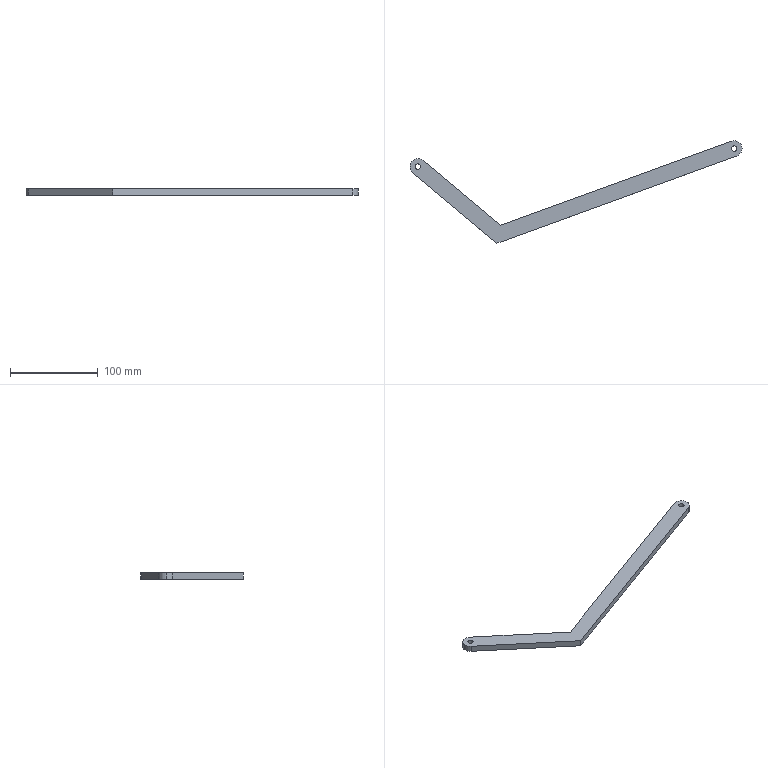Part | SolidWorks | features Extrusion 1, Fillet 1 | 1 solid | 13 faces | box 377.416 x 116.677 x 7 mm | volume 52365 mm3 | cylinder 7 | plane 6 | commonest cylinder face diameters 6 x4 18 x3
STEP:
#1=CARTESIAN_POINT('',(-3.,0.,7.));
#2=VERTEX_POINT('',#1);
#3=CARTESIAN_POINT('',(3.,0.,7.));
#4=VERTEX_POINT('',#3);
#5=CARTESIAN_POINT('',(0.,0.,7.));
#6=DIRECTION('',(0.,0.,1.));
#7=DIRECTION('',(1.,0.,0.));
#8=AXIS2_PLACEMENT_3D('',#5,#6,#7);
#9=CIRCLE('',#8,3.);
#10=EDGE_CURVE('',#2,#4,#9,.T.);
#11=ORIENTED_EDGE('',*,*,#10,.T.);
#12=CARTESIAN_POINT('',(3.,0.,0.));
#13=VERTEX_POINT('',#12);
#14=CARTESIAN_POINT('',(3.,0.,7.));
#15=DIRECTION('',(0.,0.,-1.));
#16=VECTOR('',#15,1000.);
#17=LINE('',#14,#16);
#18=EDGE_CURVE('',#4,#13,#17,.T.);
#19=ORIENTED_EDGE('',*,*,#18,.T.);
#20=CARTESIAN_POINT('',(-3.,0.,0.));
#21=VERTEX_POINT('',#20);
#22=CARTESIAN_POINT('',(0.,0.,0.));
#23=DIRECTION('',(0.,0.,1.));
#24=DIRECTION('',(1.,0.,0.));
#25=AXIS2_PLACEMENT_3D('',#22,#23,#24);
#26=CIRCLE('',#25,3.);
#27=EDGE_CURVE('',#21,#13,#26,.T.);
#28=ORIENTED_EDGE('',*,*,#27,.F.);
#29=CARTESIAN_POINT('',(-3.,0.,7.));
#30=DIRECTION('',(0.,0.,-1.));
#31=VECTOR('',#30,1000.);
#32=LINE('',#29,#31);
#33=EDGE_CURVE('',#2,#21,#32,.T.);
#34=ORIENTED_EDGE('',*,*,#33,.F.);
#35=EDGE_LOOP('',(#11,#19,#28,#34));
#36=FACE_OUTER_BOUND('',#35,.T.);
#37=CARTESIAN_POINT('',(0.,0.,7.));
#38=DIRECTION('',(0.,0.,-1.));
#39=DIRECTION('',(-1.,0.,0.));
#40=AXIS2_PLACEMENT_3D('',#37,#38,#39);
#41=CYLINDRICAL_SURFACE('',#40,3.);
#42=ADVANCED_FACE('',(#36),#41,.F.);
#43=CARTESIAN_POINT('',(356.416,20.501,7.));
#44=VERTEX_POINT('',#43);
#45=CARTESIAN_POINT('',(362.416,20.501,7.));
#46=VERTEX_POINT('',#45);
#47=CARTESIAN_POINT('',(359.416,20.501,7.));
#48=DIRECTION('',(0.,0.,1.));
#49=DIRECTION('',(1.,0.,0.));
#50=AXIS2_PLACEMENT_3D('',#47,#48,#49);
#51=CIRCLE('',#50,3.);
#52=EDGE_CURVE('',#44,#46,#51,.T.);
#53=ORIENTED_EDGE('',*,*,#52,.T.);
#54=CARTESIAN_POINT('',(362.416,20.501,0.));
#55=VERTEX_POINT('',#54);
#56=CARTESIAN_POINT('',(362.416,20.501,7.));
#57=DIRECTION('',(0.,0.,-1.));
#58=VECTOR('',#57,1000.);
#59=LINE('',#56,#58);
#60=EDGE_CURVE('',#46,#55,#59,.T.);
#61=ORIENTED_EDGE('',*,*,#60,.T.);
#62=CARTESIAN_POINT('',(356.416,20.501,0.));
#63=VERTEX_POINT('',#62);
#64=CARTESIAN_POINT('',(359.416,20.501,0.));
#65=DIRECTION('',(0.,0.,1.));
#66=DIRECTION('',(1.,0.,0.));
#67=AXIS2_PLACEMENT_3D('',#64,#65,#66);
#68=CIRCLE('',#67,3.);
#69=EDGE_CURVE('',#63,#55,#68,.T.);
#70=ORIENTED_EDGE('',*,*,#69,.F.);
#71=CARTESIAN_POINT('',(356.416,20.501,7.));
#72=DIRECTION('',(0.,0.,-1.));
#73=VECTOR('',#72,1000.);
#74=LINE('',#71,#73);
#75=EDGE_CURVE('',#44,#63,#74,.T.);
#76=ORIENTED_EDGE('',*,*,#75,.F.);
#77=EDGE_LOOP('',(#53,#61,#70,#76));
#78=FACE_OUTER_BOUND('',#77,.T.);
#79=CARTESIAN_POINT('',(359.416,20.501,7.));
#80=DIRECTION('',(0.,0.,-1.));
#81=DIRECTION('',(-1.,0.,0.));
#82=AXIS2_PLACEMENT_3D('',#79,#80,#81);
#83=CYLINDRICAL_SURFACE('',#82,3.);
#84=ADVANCED_FACE('',(#78),#83,.F.);
#85=CARTESIAN_POINT('',(-9.,0.,7.));
#86=VERTEX_POINT('',#85);
#87=CARTESIAN_POINT('',(-5.785,-6.894,7.));
#88=VERTEX_POINT('',#87);
#89=CARTESIAN_POINT('',(0.,0.,7.));
#90=DIRECTION('',(0.,0.,1.));
#91=DIRECTION('',(1.,0.,0.));
#92=AXIS2_PLACEMENT_3D('',#89,#90,#91);
#93=CIRCLE('',#92,9.);
#94=EDGE_CURVE('',#86,#88,#93,.T.);
#95=ORIENTED_EDGE('',*,*,#94,.F.);
#96=CARTESIAN_POINT('',(-9.,0.,0.));
#97=VERTEX_POINT('',#96);
#98=CARTESIAN_POINT('',(-9.,0.,7.));
#99=DIRECTION('',(0.,0.,-1.));
#100=VECTOR('',#99,1000.);
#101=LINE('',#98,#100);
#102=EDGE_CURVE('',#86,#97,#101,.T.);
#103=ORIENTED_EDGE('',*,*,#102,.T.);
#104=CARTESIAN_POINT('',(-5.785,-6.894,0.));
#105=VERTEX_POINT('',#104);
#106=CARTESIAN_POINT('',(0.,0.,0.));
#107=DIRECTION('',(0.,0.,1.));
#108=DIRECTION('',(1.,0.,0.));
#109=AXIS2_PLACEMENT_3D('',#106,#107,#108);
#110=CIRCLE('',#109,9.);
#111=EDGE_CURVE('',#97,#105,#110,.T.);
#112=ORIENTED_EDGE('',*,*,#111,.T.);
#113=CARTESIAN_POINT('',(-5.785,-6.894,7.));
#114=DIRECTION('',(0.,0.,-1.));
#115=VECTOR('',#114,1000.);
#116=LINE('',#113,#115);
#117=EDGE_CURVE('',#88,#105,#116,.T.);
#118=ORIENTED_EDGE('',*,*,#117,.F.);
#119=EDGE_LOOP('',(#95,#103,#112,#118));
#120=FACE_OUTER_BOUND('',#119,.T.);
#121=CARTESIAN_POINT('',(0.,0.,7.));
#122=DIRECTION('',(0.,0.,-1.));
#123=DIRECTION('',(-1.,0.,0.));
#124=AXIS2_PLACEMENT_3D('',#121,#122,#123);
#125=CYLINDRICAL_SURFACE('',#124,9.);
#126=ADVANCED_FACE('',(#120),#125,.T.);
#127=ORIENTED_EDGE('',*,*,#52,.F.);
#128=CARTESIAN_POINT('',(359.416,20.501,7.));
#129=DIRECTION('',(0.,0.,1.));
#130=DIRECTION('',(1.,0.,0.));
#131=AXIS2_PLACEMENT_3D('',#128,#129,#130);
#132=CIRCLE('',#131,3.);
#133=EDGE_CURVE('',#46,#44,#132,.T.);
#134=ORIENTED_EDGE('',*,*,#133,.F.);
#135=EDGE_LOOP('',(#127,#134));
#136=FACE_BOUND('',#135,.T.);
#137=CARTESIAN_POINT('',(362.494,12.044,7.));
#138=VERTEX_POINT('',#137);
#139=CARTESIAN_POINT('',(356.338,28.959,7.));
#140=VERTEX_POINT('',#139);
#141=CARTESIAN_POINT('',(359.416,20.501,7.));
#142=DIRECTION('',(0.,0.,1.));
#143=DIRECTION('',(1.,0.,0.));
#144=AXIS2_PLACEMENT_3D('',#141,#142,#143);
#145=CIRCLE('',#144,9.);
#146=EDGE_CURVE('',#138,#140,#145,.T.);
#147=ORIENTED_EDGE('',*,*,#146,.T.);
#148=CARTESIAN_POINT('',(93.5,-66.707,7.));
#149=VERTEX_POINT('',#148);
#150=CARTESIAN_POINT('',(356.338,28.959,7.));
#151=DIRECTION('',(-0.9397,-0.342,0.));
#152=VECTOR('',#151,1000.);
#153=LINE('',#150,#152);
#154=EDGE_CURVE('',#140,#149,#153,.T.);
#155=ORIENTED_EDGE('',*,*,#154,.T.);
#156=CARTESIAN_POINT('',(5.785,6.894,7.));
#157=VERTEX_POINT('',#156);
#158=CARTESIAN_POINT('',(5.785,6.894,7.));
#159=DIRECTION('',(-0.766,0.6428,0.));
#160=VECTOR('',#159,1000.);
#161=LINE('',#158,#160);
#162=EDGE_CURVE('',#149,#157,#161,.T.);
#163=ORIENTED_EDGE('',*,*,#162,.T.);
#164=CARTESIAN_POINT('',(0.,0.,7.));
#165=DIRECTION('',(0.,0.,1.));
#166=DIRECTION('',(1.,0.,0.));
#167=AXIS2_PLACEMENT_3D('',#164,#165,#166);
#168=CIRCLE('',#167,9.);
#169=EDGE_CURVE('',#157,#86,#168,.T.);
#170=ORIENTED_EDGE('',*,*,#169,.T.);
#171=ORIENTED_EDGE('',*,*,#94,.T.);
#172=CARTESIAN_POINT('',(89.89,-87.176,7.));
#173=VERTEX_POINT('',#172);
#174=CARTESIAN_POINT('',(-5.785,-6.894,7.));
#175=DIRECTION('',(0.766,-0.6428,0.));
#176=VECTOR('',#175,1000.);
#177=LINE('',#174,#176);
#178=EDGE_CURVE('',#88,#173,#177,.T.);
#179=ORIENTED_EDGE('',*,*,#178,.T.);
#180=CARTESIAN_POINT('',(362.494,12.044,7.));
#181=DIRECTION('',(0.9397,0.342,0.));
#182=VECTOR('',#181,1000.);
#183=LINE('',#180,#182);
#184=EDGE_CURVE('',#173,#138,#183,.T.);
#185=ORIENTED_EDGE('',*,*,#184,.T.);
#186=EDGE_LOOP('',(#147,#155,#163,#170,#171,#179,#185));
#187=FACE_OUTER_BOUND('',#186,.T.);
#188=ORIENTED_EDGE('',*,*,#10,.F.);
#189=CARTESIAN_POINT('',(0.,0.,7.));
#190=DIRECTION('',(0.,0.,1.));
#191=DIRECTION('',(1.,0.,0.));
#192=AXIS2_PLACEMENT_3D('',#189,#190,#191);
#193=CIRCLE('',#192,3.);
#194=EDGE_CURVE('',#4,#2,#193,.T.);
#195=ORIENTED_EDGE('',*,*,#194,.F.);
#196=EDGE_LOOP('',(#188,#195));
#197=FACE_BOUND('',#196,.T.);
#198=CARTESIAN_POINT('',(359.416,20.501,7.));
#199=DIRECTION('',(0.,0.,1.));
#200=DIRECTION('',(1.,0.,0.));
#201=AXIS2_PLACEMENT_3D('',#198,#199,#200);
#202=PLANE('',#201);
#203=ADVANCED_FACE('',(#136,#187,#197),#202,.T.);
#204=CARTESIAN_POINT('',(362.494,12.044,0.));
#205=VERTEX_POINT('',#204);
#206=CARTESIAN_POINT('',(356.338,28.959,0.));
#207=VERTEX_POINT('',#206);
#208=CARTESIAN_POINT('',(359.416,20.501,0.));
#209=DIRECTION('',(0.,0.,1.));
#210=DIRECTION('',(1.,0.,0.));
#211=AXIS2_PLACEMENT_3D('',#208,#209,#210);
#212=CIRCLE('',#211,9.);
#213=EDGE_CURVE('',#205,#207,#212,.T.);
#214=ORIENTED_EDGE('',*,*,#213,.F.);
#215=CARTESIAN_POINT('',(89.89,-87.176,0.));
#216=VERTEX_POINT('',#215);
#217=CARTESIAN_POINT('',(362.494,12.044,0.));
#218=DIRECTION('',(0.9397,0.342,0.));
#219=VECTOR('',#218,1000.);
#220=LINE('',#217,#219);
#221=EDGE_CURVE('',#216,#205,#220,.T.);
#222=ORIENTED_EDGE('',*,*,#221,.F.);
#223=CARTESIAN_POINT('',(-5.785,-6.894,0.));
#224=DIRECTION('',(0.766,-0.6428,0.));
#225=VECTOR('',#224,1000.);
#226=LINE('',#223,#225);
#227=EDGE_CURVE('',#105,#216,#226,.T.);
#228=ORIENTED_EDGE('',*,*,#227,.F.);
#229=ORIENTED_EDGE('',*,*,#111,.F.);
#230=CARTESIAN_POINT('',(5.785,6.894,0.));
#231=VERTEX_POINT('',#230);
#232=CARTESIAN_POINT('',(0.,0.,0.));
#233=DIRECTION('',(0.,0.,1.));
#234=DIRECTION('',(1.,0.,0.));
#235=AXIS2_PLACEMENT_3D('',#232,#233,#234);
#236=CIRCLE('',#235,9.);
#237=EDGE_CURVE('',#231,#97,#236,.T.);
#238=ORIENTED_EDGE('',*,*,#237,.F.);
#239=CARTESIAN_POINT('',(93.5,-66.707,0.));
#240=VERTEX_POINT('',#239);
#241=CARTESIAN_POINT('',(5.785,6.894,0.));
#242=DIRECTION('',(-0.766,0.6428,0.));
#243=VECTOR('',#242,1000.);
#244=LINE('',#241,#243);
#245=EDGE_CURVE('',#240,#231,#244,.T.);
#246=ORIENTED_EDGE('',*,*,#245,.F.);
#247=CARTESIAN_POINT('',(356.338,28.959,0.));
#248=DIRECTION('',(-0.9397,-0.342,0.));
#249=VECTOR('',#248,1000.);
#250=LINE('',#247,#249);
#251=EDGE_CURVE('',#207,#240,#250,.T.);
#252=ORIENTED_EDGE('',*,*,#251,.F.);
#253=EDGE_LOOP('',(#214,#222,#228,#229,#238,#246,#252));
#254=FACE_OUTER_BOUND('',#253,.T.);
#255=ORIENTED_EDGE('',*,*,#69,.T.);
#256=CARTESIAN_POINT('',(359.416,20.501,0.));
#257=DIRECTION('',(0.,0.,1.));
#258=DIRECTION('',(1.,0.,0.));
#259=AXIS2_PLACEMENT_3D('',#256,#257,#258);
#260=CIRCLE('',#259,3.);
#261=EDGE_CURVE('',#55,#63,#260,.T.);
#262=ORIENTED_EDGE('',*,*,#261,.T.);
#263=EDGE_LOOP('',(#255,#262));
#264=FACE_BOUND('',#263,.T.);
#265=ORIENTED_EDGE('',*,*,#27,.T.);
#266=CARTESIAN_POINT('',(0.,0.,0.));
#267=DIRECTION('',(0.,0.,1.));
#268=DIRECTION('',(1.,0.,0.));
#269=AXIS2_PLACEMENT_3D('',#266,#267,#268);
#270=CIRCLE('',#269,3.);
#271=EDGE_CURVE('',#13,#21,#270,.T.);
#272=ORIENTED_EDGE('',*,*,#271,.T.);
#273=EDGE_LOOP('',(#265,#272));
#274=FACE_BOUND('',#273,.T.);
#275=CARTESIAN_POINT('',(359.416,20.501,0.));
#276=DIRECTION('',(0.,0.,1.));
#277=DIRECTION('',(1.,0.,0.));
#278=AXIS2_PLACEMENT_3D('',#275,#276,#277);
#279=PLANE('',#278);
#280=ADVANCED_FACE('',(#254,#264,#274),#279,.F.);
#281=ORIENTED_EDGE('',*,*,#213,.T.);
#282=CARTESIAN_POINT('',(356.338,28.959,7.));
#283=DIRECTION('',(0.,0.,-1.));
#284=VECTOR('',#283,1000.);
#285=LINE('',#282,#284);
#286=EDGE_CURVE('',#140,#207,#285,.T.);
#287=ORIENTED_EDGE('',*,*,#286,.F.);
#288=ORIENTED_EDGE('',*,*,#146,.F.);
#289=CARTESIAN_POINT('',(362.494,12.044,7.));
#290=DIRECTION('',(0.,0.,-1.));
#291=VECTOR('',#290,1000.);
#292=LINE('',#289,#291);
#293=EDGE_CURVE('',#138,#205,#292,.T.);
#294=ORIENTED_EDGE('',*,*,#293,.T.);
#295=EDGE_LOOP('',(#281,#287,#288,#294));
#296=FACE_OUTER_BOUND('',#295,.T.);
#297=CARTESIAN_POINT('',(359.416,20.501,7.));
#298=DIRECTION('',(0.,0.,-1.));
#299=DIRECTION('',(-1.,0.,0.));
#300=AXIS2_PLACEMENT_3D('',#297,#298,#299);
#301=CYLINDRICAL_SURFACE('',#300,9.);
#302=ADVANCED_FACE('',(#296),#301,.T.);
#303=ORIENTED_EDGE('',*,*,#251,.T.);
#304=CARTESIAN_POINT('',(93.5,-66.707,7.));
#305=DIRECTION('',(0.,0.,-1.));
#306=VECTOR('',#305,1000.);
#307=LINE('',#304,#306);
#308=EDGE_CURVE('',#149,#240,#307,.T.);
#309=ORIENTED_EDGE('',*,*,#308,.F.);
#310=ORIENTED_EDGE('',*,*,#154,.F.);
#311=ORIENTED_EDGE('',*,*,#286,.T.);
#312=EDGE_LOOP('',(#303,#309,#310,#311));
#313=FACE_OUTER_BOUND('',#312,.T.);
#314=CARTESIAN_POINT('',(356.338,28.959,7.));
#315=DIRECTION('',(0.342,-0.9397,0.));
#316=DIRECTION('',(0.9397,0.342,0.));
#317=AXIS2_PLACEMENT_3D('',#314,#315,#316);
#318=PLANE('',#317);
#319=ADVANCED_FACE('',(#313),#318,.F.);
#320=ORIENTED_EDGE('',*,*,#245,.T.);
#321=CARTESIAN_POINT('',(5.785,6.894,7.));
#322=DIRECTION('',(0.,0.,-1.));
#323=VECTOR('',#322,1000.);
#324=LINE('',#321,#323);
#325=EDGE_CURVE('',#157,#231,#324,.T.);
#326=ORIENTED_EDGE('',*,*,#325,.F.);
#327=ORIENTED_EDGE('',*,*,#162,.F.);
#328=ORIENTED_EDGE('',*,*,#308,.T.);
#329=EDGE_LOOP('',(#320,#326,#327,#328));
#330=FACE_OUTER_BOUND('',#329,.T.);
#331=CARTESIAN_POINT('',(5.785,6.894,7.));
#332=DIRECTION('',(-0.6428,-0.766,0.));
#333=DIRECTION('',(0.766,-0.6428,0.));
#334=AXIS2_PLACEMENT_3D('',#331,#332,#333);
#335=PLANE('',#334);
#336=ADVANCED_FACE('',(#330),#335,.F.);
#337=ORIENTED_EDGE('',*,*,#102,.F.);
#338=ORIENTED_EDGE('',*,*,#169,.F.);
#339=ORIENTED_EDGE('',*,*,#325,.T.);
#340=ORIENTED_EDGE('',*,*,#237,.T.);
#341=EDGE_LOOP('',(#337,#338,#339,#340));
#342=FACE_OUTER_BOUND('',#341,.T.);
#343=CARTESIAN_POINT('',(0.,0.,7.));
#344=DIRECTION('',(0.,0.,-1.));
#345=DIRECTION('',(-1.,0.,0.));
#346=AXIS2_PLACEMENT_3D('',#343,#344,#345);
#347=CYLINDRICAL_SURFACE('',#346,9.);
#348=ADVANCED_FACE('',(#342),#347,.T.);
#349=ORIENTED_EDGE('',*,*,#227,.T.);
#350=CARTESIAN_POINT('',(89.89,-87.176,7.));
#351=DIRECTION('',(0.,0.,-1.));
#352=VECTOR('',#351,1000.);
#353=LINE('',#350,#352);
#354=EDGE_CURVE('',#173,#216,#353,.T.);
#355=ORIENTED_EDGE('',*,*,#354,.F.);
#356=ORIENTED_EDGE('',*,*,#178,.F.);
#357=ORIENTED_EDGE('',*,*,#117,.T.);
#358=EDGE_LOOP('',(#349,#355,#356,#357));
#359=FACE_OUTER_BOUND('',#358,.T.);
#360=CARTESIAN_POINT('',(-5.785,-6.894,7.));
#361=DIRECTION('',(0.6428,0.766,0.));
#362=DIRECTION('',(-0.766,0.6428,0.));
#363=AXIS2_PLACEMENT_3D('',#360,#361,#362);
#364=PLANE('',#363);
#365=ADVANCED_FACE('',(#359),#364,.F.);
#366=ORIENTED_EDGE('',*,*,#221,.T.);
#367=ORIENTED_EDGE('',*,*,#293,.F.);
#368=ORIENTED_EDGE('',*,*,#184,.F.);
#369=ORIENTED_EDGE('',*,*,#354,.T.);
#370=EDGE_LOOP('',(#366,#367,#368,#369));
#371=FACE_OUTER_BOUND('',#370,.T.);
#372=CARTESIAN_POINT('',(362.494,12.044,7.));
#373=DIRECTION('',(-0.342,0.9397,0.));
#374=DIRECTION('',(-0.9397,-0.342,0.));
#375=AXIS2_PLACEMENT_3D('',#372,#373,#374);
#376=PLANE('',#375);
#377=ADVANCED_FACE('',(#371),#376,.F.);
#378=ORIENTED_EDGE('',*,*,#60,.F.);
#379=ORIENTED_EDGE('',*,*,#133,.T.);
#380=ORIENTED_EDGE('',*,*,#75,.T.);
#381=ORIENTED_EDGE('',*,*,#261,.F.);
#382=EDGE_LOOP('',(#378,#379,#380,#381));
#383=FACE_OUTER_BOUND('',#382,.T.);
#384=CARTESIAN_POINT('',(359.416,20.501,7.));
#385=DIRECTION('',(0.,0.,-1.));
#386=DIRECTION('',(-1.,0.,0.));
#387=AXIS2_PLACEMENT_3D('',#384,#385,#386);
#388=CYLINDRICAL_SURFACE('',#387,3.);
#389=ADVANCED_FACE('',(#383),#388,.F.);
#390=ORIENTED_EDGE('',*,*,#18,.F.);
#391=ORIENTED_EDGE('',*,*,#194,.T.);
#392=ORIENTED_EDGE('',*,*,#33,.T.);
#393=ORIENTED_EDGE('',*,*,#271,.F.);
#394=EDGE_LOOP('',(#390,#391,#392,#393));
#395=FACE_OUTER_BOUND('',#394,.T.);
#396=CARTESIAN_POINT('',(0.,0.,7.));
#397=DIRECTION('',(0.,0.,-1.));
#398=DIRECTION('',(-1.,0.,0.));
#399=AXIS2_PLACEMENT_3D('',#396,#397,#398);
#400=CYLINDRICAL_SURFACE('',#399,3.);
#401=ADVANCED_FACE('',(#395),#400,.F.);
#402=CLOSED_SHELL('',(#42,#84,#126,#203,#280,#302,#319,#336,#348,#365,#377,#389,#401));
#403=MANIFOLD_SOLID_BREP('',#402);
#404=CARTESIAN_POINT('',(0.,0.,0.));
#405=DIRECTION('',(0.,0.,1.));
#406=DIRECTION('',(1.,0.,0.));
#407=AXIS2_PLACEMENT_3D('',#404,#405,#406);
#408=(LENGTH_UNIT()NAMED_UNIT(*)SI_UNIT(.MILLI.,.METRE.));
#409=UNCERTAINTY_MEASURE_WITH_UNIT(LENGTH_MEASURE(0.00001),#408,'','');
#410=(NAMED_UNIT(*)PLANE_ANGLE_UNIT()SI_UNIT($,.RADIAN.));
#411=(NAMED_UNIT(*)SI_UNIT($,.STERADIAN.)SOLID_ANGLE_UNIT());
#412=(GEOMETRIC_REPRESENTATION_CONTEXT(3)GLOBAL_UNCERTAINTY_ASSIGNED_CONTEXT((#409))GLOBAL_UNIT_ASSIGNED_CONTEXT((#408,#410,#411))REPRESENTATION_CONTEXT('',''));
#413=ADVANCED_BREP_SHAPE_REPRESENTATION('',(#403,#407),#412);